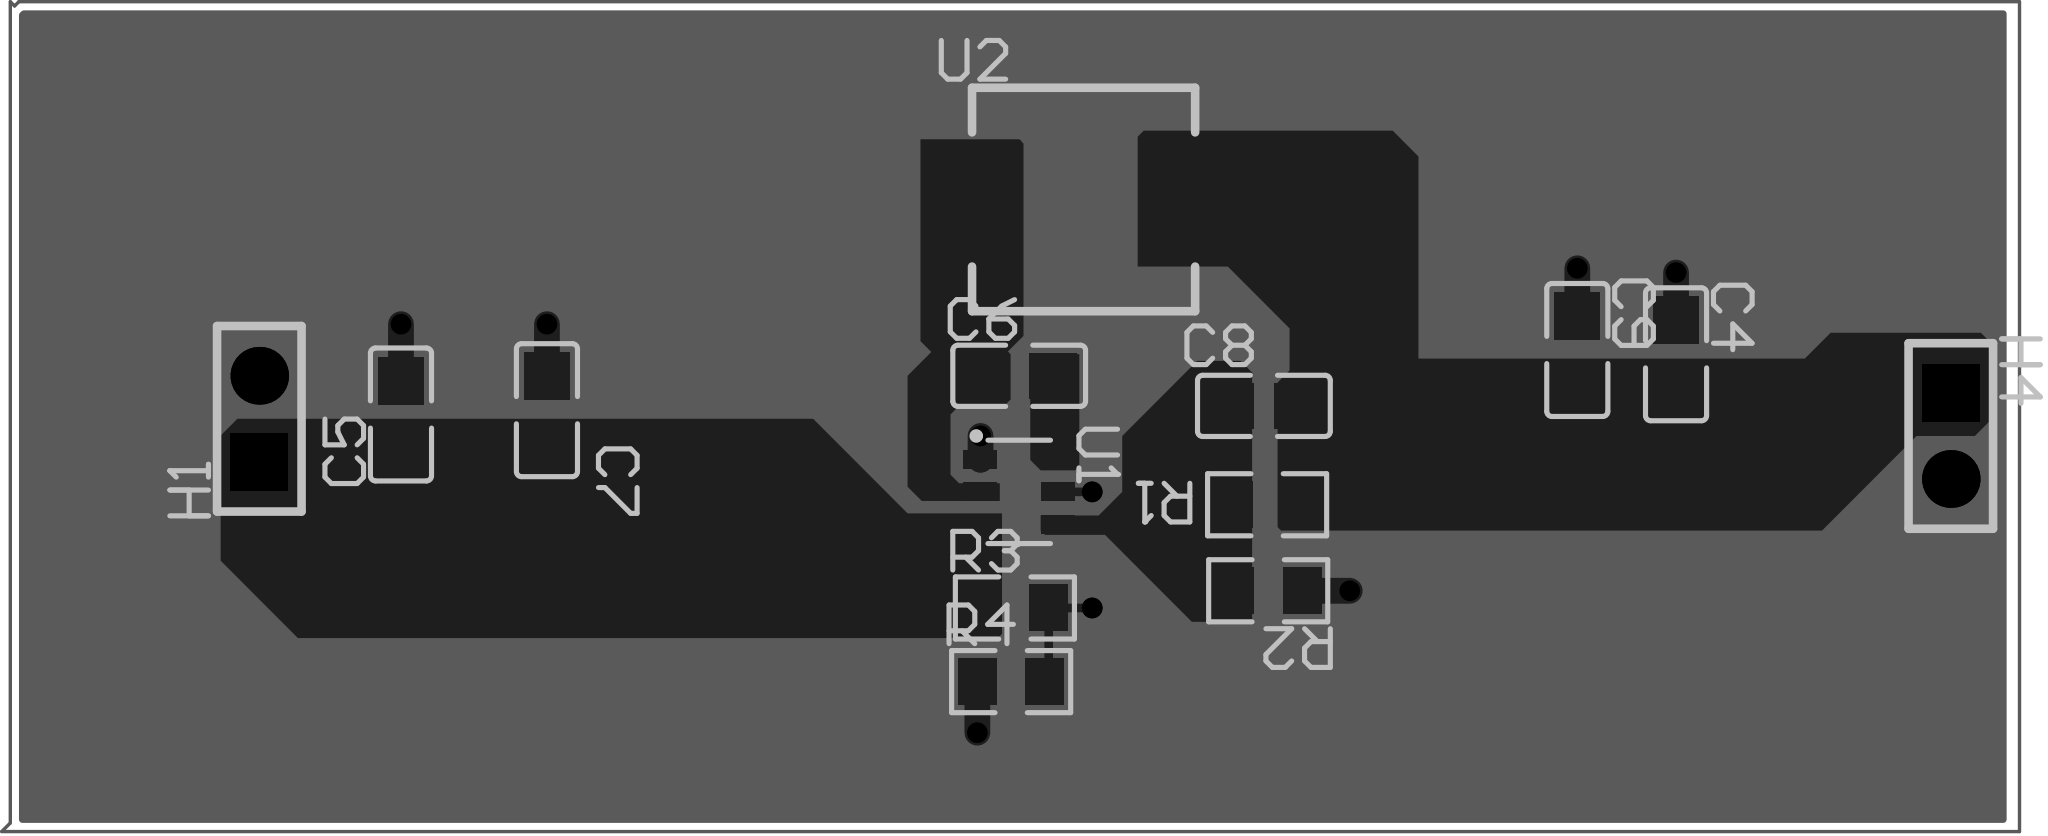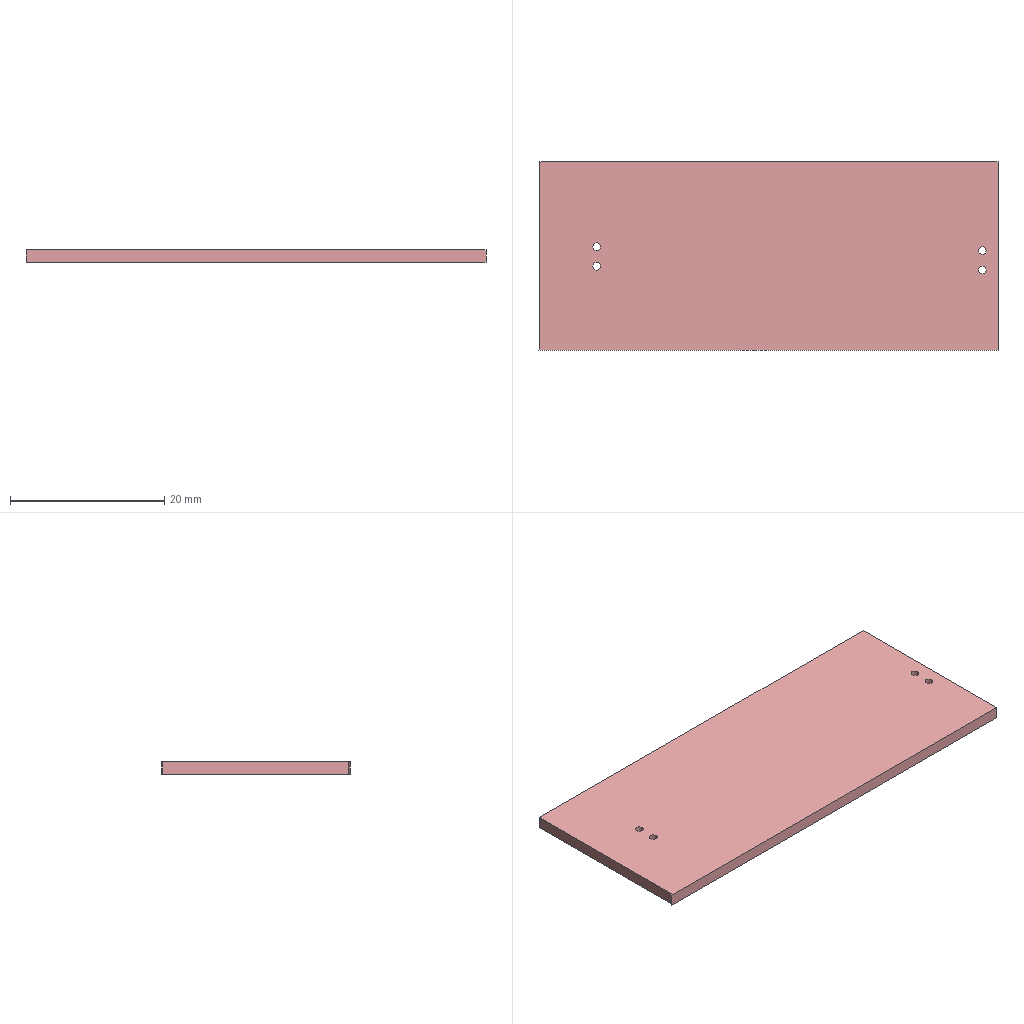Circuit board layout | Altium Designer | box 59.7 x 24.5 x 1.6 mm
Layer stack:
# Altium Designer layer stack of  (unit mm; dielectric type: 0 none, 1 core, 2 prepreg, 3 surface material)
index,name,kind,layer,copper_thickness_mm,dielectric_type,dielectric_thickness_mm,dielectric_material,dielectric_constant
0,Top Paste Mask Layer,other,,,,,,
1,Top Silkscreen Layer,other,,,,,,
2,Top Solder Mask Layer,dielectric,,,3,0.01,,3.3
3,Top Layer,copper,Top Layer,0.035,,,,
4,Dielectric1,dielectric,,,3,1.51,FR4,4.5
5,Bottom Layer,copper,Bottom Layer,0.035,,,,
6,Bottom Solder Mask Layer,dielectric,,,3,0.01,,3.3
7,Bottom Silkscreen Layer,other,,,,,,
8,Bottom Paste Mask Layer,other,,,,,,
# drill layer pairs: low layer,high layer
drill_pair,Top Layer,Bottom Layer
Part placement:
Designator,Comment,Layer,Footprint,Center-X(mm),Center-Y(mm),Rotation
C4,22uF,TopLayer,C0805,125.857,90.805,270
C5,10uF,TopLayer,C0805,88.138,89.027,90
C6,100nF,TopLayer,C0805,106.426,90.17,0
H1,电源输入,TopLayer,HDR-TH_2P-P2.54-V-F,83.947,88.9,90
H4,电源输出,TopLayer,HDR-TH_2P-P2.54-V-F,133.985,88.392,270
R1,100k,TopLayer,R0805,113.76,86.36,0
R2,13300,TopLayer,R0805,113.792,83.82,180
R3,511k,TopLayer,R0805,106.299,83.312,0
R4,105K,TopLayer,R0805,106.188,81.137,0
U1,GD30DC1354,TopLayer,SOT-23-6_L2.9-W1.7-P0.95-LS2.8-BL,106.426,86.741,270
C7,0.1uF,TopLayer,C0805,92.456,89.154,270
C8,75pF,TopLayer,C0805,113.665,89.281,0
C9,22uF,TopLayer,C0805,122.936,90.932,270
U2,15uH,TopLayer,IND-SMD_L6.6-W6.6,108.331,95.377,0
Pad and via stacks:
# Altium Designer via and pad stacks of  (unit mm). Each distinct definition once, with the count of objects using it.
# via: kind,start_layer,end_layer,hole_mm,diameter_mm,mode(0 simple;1 top-mid-bottom;2 full stack),diameter_per_layer,count,example_net
# pad: kind,layer,hole_mm,hole_type(0 round;1 square;2 slot),plating,top_size,top_shape(1 round;2 rect;3 octagon;9 rounded rect),mid_size,bottom_size,mode,footprint,size_per_layer,count,example
pad,Top Layer,0,0,plated,1.41x1.35,2,1.41x1.35,1.41x1.35,0,C0805,,12,C4.2
pad,Top Layer,0,0,plated,1.133x1.377,2,1.133x1.377,1.133x1.377,0,R0805,,8,R1.2
pad,Top Layer,0,0,plated,0.532x0.99,2,0.532x0.99,0.532x0.99,0,SOT-23-6_L2.9-W1.7-P0.95-LS2.8-BL,,6,U1.1
pad,Top Layer,0,0,plated,2.35x3.5,2,2.35x3.5,2.35x3.5,0,IND-SMD_L6.6-W6.6,,2,U2.1
pad,Multi-Layer,1,0,plated,1.7x1.7,2,1.7x1.7,1.7x1.7,0,HDR-TH_2P-P2.54-V-F,,2,H1.1
pad,Multi-Layer,1,0,plated,1.7x1.7,1,1.7x1.7,1.7x1.7,0,HDR-TH_2P-P2.54-V-F,,2,H1.2
via,Top Layer,Bottom Layer,0.3048,0.61,0,,9,$1N1606
Copper pours:
name,layer,net,type(0 solid;1 hatched;2 none)
Bottom Layer-GND,Bottom Layer,GND,0